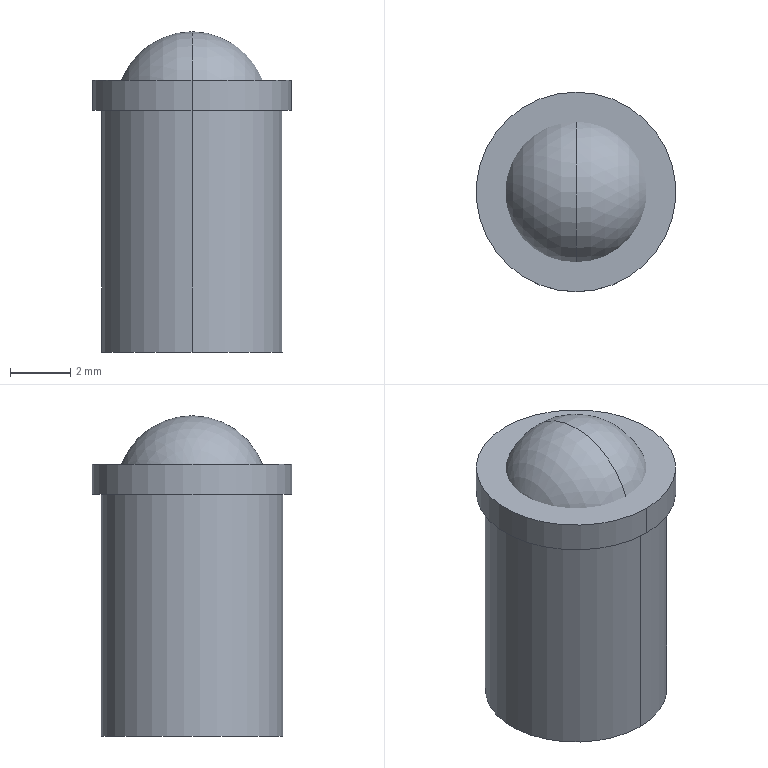Part | STEP file | 22DDSceondZAL02-M6_Default | 2 solids | 9 faces | box 6.6 x 6.6 x 10.6 mm | volume 325.856 mm3 | cylinder 4 | plane 3 | sphere 2 | commonest cylinder face diameters 6 x2 6.6 x2
STEP:
#1=CARTESIAN_POINT('',(0.,0.,0.));
#2=DIRECTION('',(0.,0.,1.));
#3=DIRECTION('',(1.,0.,0.));
#4=AXIS2_PLACEMENT_3D('',#1,#2,#3);
#5=CARTESIAN_POINT('',(0.,3.,-1.));
#6=VERTEX_POINT('',#5);
#7=CARTESIAN_POINT('',(0.,-3.,-1.));
#8=VERTEX_POINT('',#7);
#9=CARTESIAN_POINT('',(0.,0.,-1.));
#10=DIRECTION('',(0.,0.,-1.));
#11=DIRECTION('',(0.,1.,0.));
#12=AXIS2_PLACEMENT_3D('',#9,#10,#11);
#13=CIRCLE('',#12,3.);
#14=CARTESIAN_POINT('',(0.,0.,-9.));
#15=DIRECTION('',(0.,0.,-1.));
#16=DIRECTION('',(0.,1.,0.));
#17=AXIS2_PLACEMENT_3D('',#14,#15,#16);
#18=CYLINDRICAL_SURFACE('',#17,3.);
#19=CARTESIAN_POINT('',(0.,-8.));
#20=DIRECTION('',(1.,0.));
#21=VECTOR('',#20,1.);
#22=LINE('',#19,#21);
#23=(GEOMETRIC_REPRESENTATION_CONTEXT(2)PARAMETRIC_REPRESENTATION_CONTEXT()REPRESENTATION_CONTEXT('',''));
#24=DEFINITIONAL_REPRESENTATION('',(#22),#23);
#25=PCURVE('',#18,#24);
#26=CARTESIAN_POINT('',(0.,3.3,-1.));
#27=DIRECTION('',(0.,0.,-1.));
#28=DIRECTION('',(0.,1.,0.));
#29=AXIS2_PLACEMENT_3D('',#26,#27,#28);
#30=PLANE('',#29);
#31=CARTESIAN_POINT('',(-3.3,0.));
#32=DIRECTION('',(1.,0.));
#33=AXIS2_PLACEMENT_2D('',#31,#32);
#34=CIRCLE('',#33,3.);
#35=(GEOMETRIC_REPRESENTATION_CONTEXT(2)PARAMETRIC_REPRESENTATION_CONTEXT()REPRESENTATION_CONTEXT('',''));
#36=DEFINITIONAL_REPRESENTATION('',(#34),#35);
#37=PCURVE('',#30,#36);
#38=SURFACE_CURVE('',#13,(#25,#37),.PCURVE_S1.);
#39=EDGE_CURVE('',#6,#8,#38,.T.);
#40=ORIENTED_EDGE('',*,*,#39,.T.);
#41=CARTESIAN_POINT('',(0.,-3.,-9.));
#42=VERTEX_POINT('',#41);
#43=CARTESIAN_POINT('',(0.,-3.,-9.));
#44=DIRECTION('',(0.,0.,-1.));
#45=VECTOR('',#44,1.);
#46=LINE('',#43,#45);
#47=CARTESIAN_POINT('',(3.142,0.));
#48=DIRECTION('',(0.,1.));
#49=VECTOR('',#48,1.);
#50=LINE('',#47,#49);
#51=(GEOMETRIC_REPRESENTATION_CONTEXT(2)PARAMETRIC_REPRESENTATION_CONTEXT()REPRESENTATION_CONTEXT('',''));
#52=DEFINITIONAL_REPRESENTATION('',(#50),#51);
#53=PCURVE('',#18,#52);
#54=CARTESIAN_POINT('',(0.,0.,-9.));
#55=DIRECTION('',(0.,0.,-1.));
#56=DIRECTION('',(0.,1.,0.));
#57=AXIS2_PLACEMENT_3D('',#54,#55,#56);
#58=CYLINDRICAL_SURFACE('',#57,3.);
#59=CARTESIAN_POINT('',(3.142,0.));
#60=DIRECTION('',(0.,1.));
#61=VECTOR('',#60,1.);
#62=LINE('',#59,#61);
#63=(GEOMETRIC_REPRESENTATION_CONTEXT(2)PARAMETRIC_REPRESENTATION_CONTEXT()REPRESENTATION_CONTEXT('',''));
#64=DEFINITIONAL_REPRESENTATION('',(#62),#63);
#65=PCURVE('',#58,#64);
#66=SURFACE_CURVE('',#46,(#53,#65),.PCURVE_S1.);
#67=EDGE_CURVE('',#8,#42,#66,.T.);
#68=ORIENTED_EDGE('',*,*,#67,.T.);
#69=CARTESIAN_POINT('',(0.,3.,-9.));
#70=VERTEX_POINT('',#69);
#71=CARTESIAN_POINT('',(0.,0.,-9.));
#72=DIRECTION('',(0.,0.,-1.));
#73=DIRECTION('',(0.,1.,0.));
#74=AXIS2_PLACEMENT_3D('',#71,#72,#73);
#75=CIRCLE('',#74,3.);
#76=CARTESIAN_POINT('',(0.,0.));
#77=DIRECTION('',(1.,0.));
#78=VECTOR('',#77,1.);
#79=LINE('',#76,#78);
#80=(GEOMETRIC_REPRESENTATION_CONTEXT(2)PARAMETRIC_REPRESENTATION_CONTEXT()REPRESENTATION_CONTEXT('',''));
#81=DEFINITIONAL_REPRESENTATION('',(#79),#80);
#82=PCURVE('',#18,#81);
#83=CARTESIAN_POINT('',(0.,3.,-9.));
#84=DIRECTION('',(0.,0.,-1.));
#85=DIRECTION('',(0.,1.,0.));
#86=AXIS2_PLACEMENT_3D('',#83,#84,#85);
#87=PLANE('',#86);
#88=CARTESIAN_POINT('',(-3.,0.));
#89=DIRECTION('',(1.,0.));
#90=AXIS2_PLACEMENT_2D('',#88,#89);
#91=CIRCLE('',#90,3.);
#92=(GEOMETRIC_REPRESENTATION_CONTEXT(2)PARAMETRIC_REPRESENTATION_CONTEXT()REPRESENTATION_CONTEXT('',''));
#93=DEFINITIONAL_REPRESENTATION('',(#91),#92);
#94=PCURVE('',#87,#93);
#95=SURFACE_CURVE('',#75,(#82,#94),.PCURVE_S1.);
#96=EDGE_CURVE('',#70,#42,#95,.T.);
#97=ORIENTED_EDGE('',*,*,#96,.F.);
#98=CARTESIAN_POINT('',(0.,3.,-9.));
#99=DIRECTION('',(0.,0.,-1.));
#100=VECTOR('',#99,1.);
#101=LINE('',#98,#100);
#102=CARTESIAN_POINT('',(0.,0.));
#103=DIRECTION('',(0.,1.));
#104=VECTOR('',#103,1.);
#105=LINE('',#102,#104);
#106=(GEOMETRIC_REPRESENTATION_CONTEXT(2)PARAMETRIC_REPRESENTATION_CONTEXT()REPRESENTATION_CONTEXT('',''));
#107=DEFINITIONAL_REPRESENTATION('',(#105),#106);
#108=PCURVE('',#18,#107);
#109=CARTESIAN_POINT('',(6.283,0.));
#110=DIRECTION('',(0.,1.));
#111=VECTOR('',#110,1.);
#112=LINE('',#109,#111);
#113=(GEOMETRIC_REPRESENTATION_CONTEXT(2)PARAMETRIC_REPRESENTATION_CONTEXT()REPRESENTATION_CONTEXT('',''));
#114=DEFINITIONAL_REPRESENTATION('',(#112),#113);
#115=PCURVE('',#58,#114);
#116=SURFACE_CURVE('',#101,(#108,#115),.PCURVE_S1.);
#117=EDGE_CURVE('',#6,#70,#116,.T.);
#118=ORIENTED_EDGE('',*,*,#117,.F.);
#119=EDGE_LOOP('',(#40,#68,#97,#118));
#120=FACE_BOUND('',#119,.T.);
#121=ADVANCED_FACE('',(#120),#18,.T.);
#122=CARTESIAN_POINT('',(0.,3.3,0.));
#123=VERTEX_POINT('',#122);
#124=CARTESIAN_POINT('',(0.,-3.3,0.));
#125=VERTEX_POINT('',#124);
#126=CARTESIAN_POINT('',(0.,0.,0.));
#127=DIRECTION('',(0.,0.,-1.));
#128=DIRECTION('',(0.,1.,0.));
#129=AXIS2_PLACEMENT_3D('',#126,#127,#128);
#130=CIRCLE('',#129,3.3);
#131=CARTESIAN_POINT('',(0.,0.,-9.));
#132=DIRECTION('',(0.,0.,-1.));
#133=DIRECTION('',(0.,1.,0.));
#134=AXIS2_PLACEMENT_3D('',#131,#132,#133);
#135=CYLINDRICAL_SURFACE('',#134,3.3);
#136=CARTESIAN_POINT('',(0.,-9.));
#137=DIRECTION('',(1.,0.));
#138=VECTOR('',#137,1.);
#139=LINE('',#136,#138);
#140=(GEOMETRIC_REPRESENTATION_CONTEXT(2)PARAMETRIC_REPRESENTATION_CONTEXT()REPRESENTATION_CONTEXT('',''));
#141=DEFINITIONAL_REPRESENTATION('',(#139),#140);
#142=PCURVE('',#135,#141);
#143=CARTESIAN_POINT('',(0.,0.,0.));
#144=DIRECTION('',(0.,0.,1.));
#145=DIRECTION('',(0.,-1.,0.));
#146=AXIS2_PLACEMENT_3D('',#143,#144,#145);
#147=PLANE('',#146);
#148=CARTESIAN_POINT('',(-3.3,0.));
#149=CARTESIAN_POINT('',(-3.3,5.716));
#150=CARTESIAN_POINT('',(1.65,2.858));
#151=CARTESIAN_POINT('',(6.6,0.));
#152=CARTESIAN_POINT('',(1.65,-2.858));
#153=CARTESIAN_POINT('',(-3.3,-5.716));
#154=CARTESIAN_POINT('',(-3.3,0.));
#155=(BOUNDED_CURVE()B_SPLINE_CURVE(2,(#148,#149,#150,#151,#152,#153,#154),.UNSPECIFIED.,.T.,.F.)B_SPLINE_CURVE_WITH_KNOTS((1,2,2,2,2,1),(-2.094,0.,2.094,4.189,6.283,8.378),.UNSPECIFIED.)CURVE()GEOMETRIC_REPRESENTATION_ITEM()RATIONAL_B_SPLINE_CURVE((1.,0.5,1.,0.5,1.,0.5,1.))REPRESENTATION_ITEM(''));
#156=(GEOMETRIC_REPRESENTATION_CONTEXT(2)PARAMETRIC_REPRESENTATION_CONTEXT()REPRESENTATION_CONTEXT('',''));
#157=DEFINITIONAL_REPRESENTATION('',(#155),#156);
#158=PCURVE('',#147,#157);
#159=SURFACE_CURVE('',#130,(#142,#158),.PCURVE_S1.);
#160=EDGE_CURVE('',#123,#125,#159,.T.);
#161=ORIENTED_EDGE('',*,*,#160,.T.);
#162=CARTESIAN_POINT('',(0.,-3.3,-1.));
#163=VERTEX_POINT('',#162);
#164=CARTESIAN_POINT('',(0.,-3.3,-9.));
#165=DIRECTION('',(0.,0.,-1.));
#166=VECTOR('',#165,1.);
#167=LINE('',#164,#166);
#168=CARTESIAN_POINT('',(3.142,0.));
#169=DIRECTION('',(0.,1.));
#170=VECTOR('',#169,1.);
#171=LINE('',#168,#170);
#172=(GEOMETRIC_REPRESENTATION_CONTEXT(2)PARAMETRIC_REPRESENTATION_CONTEXT()REPRESENTATION_CONTEXT('',''));
#173=DEFINITIONAL_REPRESENTATION('',(#171),#172);
#174=PCURVE('',#135,#173);
#175=CARTESIAN_POINT('',(0.,0.,-9.));
#176=DIRECTION('',(0.,0.,-1.));
#177=DIRECTION('',(0.,1.,0.));
#178=AXIS2_PLACEMENT_3D('',#175,#176,#177);
#179=CYLINDRICAL_SURFACE('',#178,3.3);
#180=CARTESIAN_POINT('',(3.142,0.));
#181=DIRECTION('',(0.,1.));
#182=VECTOR('',#181,1.);
#183=LINE('',#180,#182);
#184=(GEOMETRIC_REPRESENTATION_CONTEXT(2)PARAMETRIC_REPRESENTATION_CONTEXT()REPRESENTATION_CONTEXT('',''));
#185=DEFINITIONAL_REPRESENTATION('',(#183),#184);
#186=PCURVE('',#179,#185);
#187=SURFACE_CURVE('',#167,(#174,#186),.PCURVE_S1.);
#188=EDGE_CURVE('',#125,#163,#187,.T.);
#189=ORIENTED_EDGE('',*,*,#188,.T.);
#190=CARTESIAN_POINT('',(0.,3.3,-1.));
#191=VERTEX_POINT('',#190);
#192=CARTESIAN_POINT('',(0.,0.,-1.));
#193=DIRECTION('',(0.,0.,-1.));
#194=DIRECTION('',(0.,1.,0.));
#195=AXIS2_PLACEMENT_3D('',#192,#193,#194);
#196=CIRCLE('',#195,3.3);
#197=CARTESIAN_POINT('',(0.,-8.));
#198=DIRECTION('',(1.,0.));
#199=VECTOR('',#198,1.);
#200=LINE('',#197,#199);
#201=(GEOMETRIC_REPRESENTATION_CONTEXT(2)PARAMETRIC_REPRESENTATION_CONTEXT()REPRESENTATION_CONTEXT('',''));
#202=DEFINITIONAL_REPRESENTATION('',(#200),#201);
#203=PCURVE('',#135,#202);
#204=CARTESIAN_POINT('',(-3.3,0.));
#205=DIRECTION('',(1.,0.));
#206=AXIS2_PLACEMENT_2D('',#204,#205);
#207=CIRCLE('',#206,3.3);
#208=(GEOMETRIC_REPRESENTATION_CONTEXT(2)PARAMETRIC_REPRESENTATION_CONTEXT()REPRESENTATION_CONTEXT('',''));
#209=DEFINITIONAL_REPRESENTATION('',(#207),#208);
#210=PCURVE('',#30,#209);
#211=SURFACE_CURVE('',#196,(#203,#210),.PCURVE_S1.);
#212=EDGE_CURVE('',#191,#163,#211,.T.);
#213=ORIENTED_EDGE('',*,*,#212,.F.);
#214=CARTESIAN_POINT('',(0.,3.3,-9.));
#215=DIRECTION('',(0.,0.,-1.));
#216=VECTOR('',#215,1.);
#217=LINE('',#214,#216);
#218=CARTESIAN_POINT('',(0.,0.));
#219=DIRECTION('',(0.,1.));
#220=VECTOR('',#219,1.);
#221=LINE('',#218,#220);
#222=(GEOMETRIC_REPRESENTATION_CONTEXT(2)PARAMETRIC_REPRESENTATION_CONTEXT()REPRESENTATION_CONTEXT('',''));
#223=DEFINITIONAL_REPRESENTATION('',(#221),#222);
#224=PCURVE('',#135,#223);
#225=CARTESIAN_POINT('',(6.283,0.));
#226=DIRECTION('',(0.,1.));
#227=VECTOR('',#226,1.);
#228=LINE('',#225,#227);
#229=(GEOMETRIC_REPRESENTATION_CONTEXT(2)PARAMETRIC_REPRESENTATION_CONTEXT()REPRESENTATION_CONTEXT('',''));
#230=DEFINITIONAL_REPRESENTATION('',(#228),#229);
#231=PCURVE('',#179,#230);
#232=SURFACE_CURVE('',#217,(#224,#231),.PCURVE_S1.);
#233=EDGE_CURVE('',#123,#191,#232,.T.);
#234=ORIENTED_EDGE('',*,*,#233,.F.);
#235=EDGE_LOOP('',(#161,#189,#213,#234));
#236=FACE_BOUND('',#235,.T.);
#237=ADVANCED_FACE('',(#236),#135,.T.);
#238=ORIENTED_EDGE('',*,*,#188,.F.);
#239=CARTESIAN_POINT('',(0.,0.,0.));
#240=DIRECTION('',(0.,0.,-1.));
#241=DIRECTION('',(0.,1.,0.));
#242=AXIS2_PLACEMENT_3D('',#239,#240,#241);
#243=CIRCLE('',#242,3.3);
#244=CARTESIAN_POINT('',(0.,-9.));
#245=DIRECTION('',(1.,0.));
#246=VECTOR('',#245,1.);
#247=LINE('',#244,#246);
#248=(GEOMETRIC_REPRESENTATION_CONTEXT(2)PARAMETRIC_REPRESENTATION_CONTEXT()REPRESENTATION_CONTEXT('',''));
#249=DEFINITIONAL_REPRESENTATION('',(#247),#248);
#250=PCURVE('',#179,#249);
#251=CARTESIAN_POINT('',(-3.3,0.));
#252=CARTESIAN_POINT('',(-3.3,5.716));
#253=CARTESIAN_POINT('',(1.65,2.858));
#254=CARTESIAN_POINT('',(6.6,0.));
#255=CARTESIAN_POINT('',(1.65,-2.858));
#256=CARTESIAN_POINT('',(-3.3,-5.716));
#257=CARTESIAN_POINT('',(-3.3,0.));
#258=(BOUNDED_CURVE()B_SPLINE_CURVE(2,(#251,#252,#253,#254,#255,#256,#257),.UNSPECIFIED.,.T.,.F.)B_SPLINE_CURVE_WITH_KNOTS((1,2,2,2,2,1),(-2.094,0.,2.094,4.189,6.283,8.378),.UNSPECIFIED.)CURVE()GEOMETRIC_REPRESENTATION_ITEM()RATIONAL_B_SPLINE_CURVE((1.,0.5,1.,0.5,1.,0.5,1.))REPRESENTATION_ITEM(''));
#259=(GEOMETRIC_REPRESENTATION_CONTEXT(2)PARAMETRIC_REPRESENTATION_CONTEXT()REPRESENTATION_CONTEXT('',''));
#260=DEFINITIONAL_REPRESENTATION('',(#258),#259);
#261=PCURVE('',#147,#260);
#262=SURFACE_CURVE('',#243,(#250,#261),.PCURVE_S1.);
#263=EDGE_CURVE('',#125,#123,#262,.T.);
#264=ORIENTED_EDGE('',*,*,#263,.T.);
#265=ORIENTED_EDGE('',*,*,#233,.T.);
#266=CARTESIAN_POINT('',(0.,0.,-1.));
#267=DIRECTION('',(0.,0.,-1.));
#268=DIRECTION('',(0.,1.,0.));
#269=AXIS2_PLACEMENT_3D('',#266,#267,#268);
#270=CIRCLE('',#269,3.3);
#271=CARTESIAN_POINT('',(0.,-8.));
#272=DIRECTION('',(1.,0.));
#273=VECTOR('',#272,1.);
#274=LINE('',#271,#273);
#275=(GEOMETRIC_REPRESENTATION_CONTEXT(2)PARAMETRIC_REPRESENTATION_CONTEXT()REPRESENTATION_CONTEXT('',''));
#276=DEFINITIONAL_REPRESENTATION('',(#274),#275);
#277=PCURVE('',#179,#276);
#278=CARTESIAN_POINT('',(-3.3,0.));
#279=DIRECTION('',(1.,0.));
#280=AXIS2_PLACEMENT_2D('',#278,#279);
#281=CIRCLE('',#280,3.3);
#282=(GEOMETRIC_REPRESENTATION_CONTEXT(2)PARAMETRIC_REPRESENTATION_CONTEXT()REPRESENTATION_CONTEXT('',''));
#283=DEFINITIONAL_REPRESENTATION('',(#281),#282);
#284=PCURVE('',#30,#283);
#285=SURFACE_CURVE('',#270,(#277,#284),.PCURVE_S1.);
#286=EDGE_CURVE('',#163,#191,#285,.T.);
#287=ORIENTED_EDGE('',*,*,#286,.F.);
#288=EDGE_LOOP('',(#238,#264,#265,#287));
#289=FACE_BOUND('',#288,.T.);
#290=ADVANCED_FACE('',(#289),#179,.T.);
#291=ORIENTED_EDGE('',*,*,#212,.T.);
#292=ORIENTED_EDGE('',*,*,#286,.T.);
#293=EDGE_LOOP('',(#291,#292));
#294=FACE_BOUND('',#293,.T.);
#295=ORIENTED_EDGE('',*,*,#39,.F.);
#296=CARTESIAN_POINT('',(0.,0.,-1.));
#297=DIRECTION('',(0.,0.,-1.));
#298=DIRECTION('',(0.,1.,0.));
#299=AXIS2_PLACEMENT_3D('',#296,#297,#298);
#300=CIRCLE('',#299,3.);
#301=CARTESIAN_POINT('',(-3.3,0.));
#302=DIRECTION('',(1.,0.));
#303=AXIS2_PLACEMENT_2D('',#301,#302);
#304=CIRCLE('',#303,3.);
#305=(GEOMETRIC_REPRESENTATION_CONTEXT(2)PARAMETRIC_REPRESENTATION_CONTEXT()REPRESENTATION_CONTEXT('',''));
#306=DEFINITIONAL_REPRESENTATION('',(#304),#305);
#307=PCURVE('',#30,#306);
#308=CARTESIAN_POINT('',(0.,-8.));
#309=DIRECTION('',(1.,0.));
#310=VECTOR('',#309,1.);
#311=LINE('',#308,#310);
#312=(GEOMETRIC_REPRESENTATION_CONTEXT(2)PARAMETRIC_REPRESENTATION_CONTEXT()REPRESENTATION_CONTEXT('',''));
#313=DEFINITIONAL_REPRESENTATION('',(#311),#312);
#314=PCURVE('',#58,#313);
#315=SURFACE_CURVE('',#300,(#307,#314),.PCURVE_S1.);
#316=EDGE_CURVE('',#8,#6,#315,.T.);
#317=ORIENTED_EDGE('',*,*,#316,.F.);
#318=EDGE_LOOP('',(#295,#317));
#319=FACE_BOUND('',#318,.T.);
#320=ADVANCED_FACE('',(#294,#319),#30,.T.);
#321=ORIENTED_EDGE('',*,*,#67,.F.);
#322=ORIENTED_EDGE('',*,*,#316,.T.);
#323=ORIENTED_EDGE('',*,*,#117,.T.);
#324=CARTESIAN_POINT('',(0.,0.,-9.));
#325=DIRECTION('',(0.,0.,-1.));
#326=DIRECTION('',(0.,1.,0.));
#327=AXIS2_PLACEMENT_3D('',#324,#325,#326);
#328=CIRCLE('',#327,3.);
#329=CARTESIAN_POINT('',(0.,0.));
#330=DIRECTION('',(1.,0.));
#331=VECTOR('',#330,1.);
#332=LINE('',#329,#331);
#333=(GEOMETRIC_REPRESENTATION_CONTEXT(2)PARAMETRIC_REPRESENTATION_CONTEXT()REPRESENTATION_CONTEXT('',''));
#334=DEFINITIONAL_REPRESENTATION('',(#332),#333);
#335=PCURVE('',#58,#334);
#336=CARTESIAN_POINT('',(-3.,0.));
#337=DIRECTION('',(1.,0.));
#338=AXIS2_PLACEMENT_2D('',#336,#337);
#339=CIRCLE('',#338,3.);
#340=(GEOMETRIC_REPRESENTATION_CONTEXT(2)PARAMETRIC_REPRESENTATION_CONTEXT()REPRESENTATION_CONTEXT('',''));
#341=DEFINITIONAL_REPRESENTATION('',(#339),#340);
#342=PCURVE('',#87,#341);
#343=SURFACE_CURVE('',#328,(#335,#342),.PCURVE_S1.);
#344=EDGE_CURVE('',#42,#70,#343,.T.);
#345=ORIENTED_EDGE('',*,*,#344,.F.);
#346=EDGE_LOOP('',(#321,#322,#323,#345));
#347=FACE_BOUND('',#346,.T.);
#348=ADVANCED_FACE('',(#347),#58,.T.);
#349=ORIENTED_EDGE('',*,*,#96,.T.);
#350=ORIENTED_EDGE('',*,*,#344,.T.);
#351=EDGE_LOOP('',(#349,#350));
#352=FACE_BOUND('',#351,.T.);
#353=ADVANCED_FACE('',(#352),#87,.T.);
#354=ORIENTED_EDGE('',*,*,#160,.F.);
#355=ORIENTED_EDGE('',*,*,#263,.F.);
#356=EDGE_LOOP('',(#354,#355));
#357=FACE_BOUND('',#356,.T.);
#358=ADVANCED_FACE('',(#357),#147,.T.);
#359=CLOSED_SHELL('',(#121,#237,#290,#320,#348,#353,#358));
#360=MANIFOLD_SOLID_BREP('',#359);
#361=CARTESIAN_POINT('',(0.,2.5,-0.9));
#362=VERTEX_POINT('',#361);
#363=CARTESIAN_POINT('',(0.,0.,1.6));
#364=VERTEX_POINT('',#363);
#365=CARTESIAN_POINT('',(0.,0.,-0.9));
#366=DIRECTION('',(1.,0.,0.));
#367=DIRECTION('',(0.,0.,-1.));
#368=AXIS2_PLACEMENT_3D('',#365,#366,#367);
#369=CIRCLE('',#368,2.5);
#370=CARTESIAN_POINT('',(0.,0.,-0.9));
#371=DIRECTION('',(-1.,0.,0.));
#372=DIRECTION('',(0.,1.,0.));
#373=AXIS2_PLACEMENT_3D('',#370,#371,#372);
#374=SPHERICAL_SURFACE('',#373,2.5);
#375=CARTESIAN_POINT('',(7.854,0.));
#376=CARTESIAN_POINT('',(7.806,0.));
#377=CARTESIAN_POINT('',(7.711,0.));
#378=CARTESIAN_POINT('',(7.568,0.));
#379=CARTESIAN_POINT('',(7.426,0.));
#380=CARTESIAN_POINT('',(7.283,0.));
#381=CARTESIAN_POINT('',(7.14,0.));
#382=CARTESIAN_POINT('',(6.997,0.));
#383=CARTESIAN_POINT('',(6.854,0.));
#384=CARTESIAN_POINT('',(6.712,0.));
#385=CARTESIAN_POINT('',(6.569,0.));
#386=CARTESIAN_POINT('',(6.426,0.));
#387=CARTESIAN_POINT('',(6.283,0.));
#388=CARTESIAN_POINT('',(6.14,0.));
#389=CARTESIAN_POINT('',(5.998,0.));
#390=CARTESIAN_POINT('',(5.855,0.));
#391=CARTESIAN_POINT('',(5.712,0.));
#392=CARTESIAN_POINT('',(5.569,0.));
#393=CARTESIAN_POINT('',(5.426,0.));
#394=CARTESIAN_POINT('',(5.284,0.));
#395=CARTESIAN_POINT('',(5.141,0.));
#396=CARTESIAN_POINT('',(4.998,0.));
#397=CARTESIAN_POINT('',(4.855,0.));
#398=CARTESIAN_POINT('',(4.76,0.));
#399=CARTESIAN_POINT('',(4.712,0.));
#400=B_SPLINE_CURVE_WITH_KNOTS('',3,(#375,#376,#377,#378,#379,#380,#381,#382,#383,#384,#385,#386,#387,#388,#389,#390,#391,#392,#393,#394,#395,#396,#397,#398,#399),.UNSPECIFIED.,.F.,.F.,(4,1,1,1,1,1,1,1,1,1,1,1,1,1,1,1,1,1,1,1,1,1,4),(0.,0.1428,0.2856,0.4284,0.5712,0.714,0.8568,0.9996,1.142,1.285,1.428,1.571,1.714,1.856,1.999,2.142,2.285,2.428,2.57,2.713,2.856,2.999,3.142),.QUASI_UNIFORM_KNOTS.);
#401=(GEOMETRIC_REPRESENTATION_CONTEXT(2)PARAMETRIC_REPRESENTATION_CONTEXT()REPRESENTATION_CONTEXT('',''));
#402=DEFINITIONAL_REPRESENTATION('',(#400),#401);
#403=PCURVE('',#374,#402);
#404=CARTESIAN_POINT('',(0.,0.,-0.9));
#405=DIRECTION('',(-1.,0.,0.));
#406=DIRECTION('',(0.,1.,0.));
#407=AXIS2_PLACEMENT_3D('',#404,#405,#406);
#408=SPHERICAL_SURFACE('',#407,2.5);
#409=CARTESIAN_POINT('',(6.283,0.));
#410=CARTESIAN_POINT('',(6.259,0.));
#411=CARTESIAN_POINT('',(6.212,0.));
#412=CARTESIAN_POINT('',(6.14,0.));
#413=CARTESIAN_POINT('',(6.069,0.));
#414=CARTESIAN_POINT('',(5.998,0.));
#415=CARTESIAN_POINT('',(5.926,0.));
#416=CARTESIAN_POINT('',(5.855,0.));
#417=CARTESIAN_POINT('',(5.783,0.));
#418=CARTESIAN_POINT('',(5.712,0.));
#419=CARTESIAN_POINT('',(5.641,0.));
#420=CARTESIAN_POINT('',(5.569,0.));
#421=CARTESIAN_POINT('',(5.498,0.));
#422=CARTESIAN_POINT('',(5.426,0.));
#423=CARTESIAN_POINT('',(5.355,0.));
#424=CARTESIAN_POINT('',(5.284,0.));
#425=CARTESIAN_POINT('',(5.212,0.));
#426=CARTESIAN_POINT('',(5.141,0.));
#427=CARTESIAN_POINT('',(5.069,0.));
#428=CARTESIAN_POINT('',(4.998,0.));
#429=CARTESIAN_POINT('',(4.927,0.));
#430=CARTESIAN_POINT('',(4.855,0.));
#431=CARTESIAN_POINT('',(4.784,0.));
#432=CARTESIAN_POINT('',(4.736,0.));
#433=CARTESIAN_POINT('',(4.712,0.));
#434=B_SPLINE_CURVE_WITH_KNOTS('',3,(#409,#410,#411,#412,#413,#414,#415,#416,#417,#418,#419,#420,#421,#422,#423,#424,#425,#426,#427,#428,#429,#430,#431,#432,#433),.UNSPECIFIED.,.F.,.F.,(4,1,1,1,1,1,1,1,1,1,1,1,1,1,1,1,1,1,1,1,1,1,4),(1.571,1.642,1.714,1.785,1.856,1.928,1.999,2.071,2.142,2.213,2.285,2.356,2.428,2.499,2.57,2.642,2.713,2.785,2.856,2.927,2.999,3.07,3.142),.QUASI_UNIFORM_KNOTS.);
#435=(GEOMETRIC_REPRESENTATION_CONTEXT(2)PARAMETRIC_REPRESENTATION_CONTEXT()REPRESENTATION_CONTEXT('',''));
#436=DEFINITIONAL_REPRESENTATION('',(#434),#435);
#437=PCURVE('',#408,#436);
#438=SURFACE_CURVE('',#369,(#403,#437),.PCURVE_S1.);
#439=EDGE_CURVE('',#362,#364,#438,.T.);
#440=ORIENTED_EDGE('',*,*,#439,.F.);
#441=CARTESIAN_POINT('',(-2.5,0.,-0.9));
#442=VERTEX_POINT('',#441);
#443=CARTESIAN_POINT('',(0.,2.5,-0.9));
#444=CARTESIAN_POINT('',(-0.6545,2.5,-0.9));
#445=CARTESIAN_POINT('',(-1.309,2.294,-0.9));
#446=CARTESIAN_POINT('',(-1.883,1.883,-0.9));
#447=CARTESIAN_POINT('',(-2.294,1.309,-0.9));
#448=CARTESIAN_POINT('',(-2.5,0.6545,-0.9));
#449=CARTESIAN_POINT('',(-2.5,0.,-0.9));
#450=B_SPLINE_CURVE_WITH_KNOTS('',6,(#443,#444,#445,#446,#447,#448,#449),.UNSPECIFIED.,.F.,.F.,(7,7),(0.,1.571),.PIECEWISE_BEZIER_KNOTS.);
#451=CARTESIAN_POINT('',(6.283,0.));
#452=DIRECTION('',(0.,1.));
#453=VECTOR('',#452,1.);
#454=LINE('',#451,#453);
#455=(GEOMETRIC_REPRESENTATION_CONTEXT(2)PARAMETRIC_REPRESENTATION_CONTEXT()REPRESENTATION_CONTEXT('',''));
#456=DEFINITIONAL_REPRESENTATION('',(#454),#455);
#457=PCURVE('',#374,#456);
#458=CARTESIAN_POINT('',(0.,0.));
#459=DIRECTION('',(0.,1.));
#460=VECTOR('',#459,1.);
#461=LINE('',#458,#460);
#462=(GEOMETRIC_REPRESENTATION_CONTEXT(2)PARAMETRIC_REPRESENTATION_CONTEXT()REPRESENTATION_CONTEXT('',''));
#463=DEFINITIONAL_REPRESENTATION('',(#461),#462);
#464=PCURVE('',#374,#463);
#465=SEAM_CURVE('',#450,(#457,#464),.PCURVE_S1.);
#466=EDGE_CURVE('',#362,#442,#465,.T.);
#467=ORIENTED_EDGE('',*,*,#466,.T.);
#468=ORIENTED_EDGE('',*,*,#466,.F.);
#469=CARTESIAN_POINT('',(0.,0.,-3.4));
#470=VERTEX_POINT('',#469);
#471=CARTESIAN_POINT('',(0.,0.,-0.9));
#472=DIRECTION('',(1.,0.,0.));
#473=DIRECTION('',(0.,0.,-1.));
#474=AXIS2_PLACEMENT_3D('',#471,#472,#473);
#475=CIRCLE('',#474,2.5);
#476=CARTESIAN_POINT('',(1.571,0.));
#477=CARTESIAN_POINT('',(1.523,0.));
#478=CARTESIAN_POINT('',(1.428,0.));
#479=CARTESIAN_POINT('',(1.285,0.));
#480=CARTESIAN_POINT('',(1.142,0.));
#481=CARTESIAN_POINT('',(0.9996,0.));
#482=CARTESIAN_POINT('',(0.8568,0.));
#483=CARTESIAN_POINT('',(0.714,0.));
#484=CARTESIAN_POINT('',(0.5712,0.));
#485=CARTESIAN_POINT('',(0.4284,0.));
#486=CARTESIAN_POINT('',(0.2856,0.));
#487=CARTESIAN_POINT('',(0.1428,0.));
#488=CARTESIAN_POINT('',(0.,0.));
#489=CARTESIAN_POINT('',(-0.1428,0.));
#490=CARTESIAN_POINT('',(-0.2856,0.));
#491=CARTESIAN_POINT('',(-0.4284,0.));
#492=CARTESIAN_POINT('',(-0.5712,0.));
#493=CARTESIAN_POINT('',(-0.714,0.));
#494=CARTESIAN_POINT('',(-0.8568,0.));
#495=CARTESIAN_POINT('',(-0.9996,0.));
#496=CARTESIAN_POINT('',(-1.142,0.));
#497=CARTESIAN_POINT('',(-1.285,0.));
#498=CARTESIAN_POINT('',(-1.428,0.));
#499=CARTESIAN_POINT('',(-1.523,0.));
#500=CARTESIAN_POINT('',(-1.571,0.));
#501=B_SPLINE_CURVE_WITH_KNOTS('',3,(#476,#477,#478,#479,#480,#481,#482,#483,#484,#485,#486,#487,#488,#489,#490,#491,#492,#493,#494,#495,#496,#497,#498,#499,#500),.UNSPECIFIED.,.F.,.F.,(4,1,1,1,1,1,1,1,1,1,1,1,1,1,1,1,1,1,1,1,1,1,4),(0.,0.1428,0.2856,0.4284,0.5712,0.714,0.8568,0.9996,1.142,1.285,1.428,1.571,1.714,1.856,1.999,2.142,2.285,2.428,2.57,2.713,2.856,2.999,3.142),.QUASI_UNIFORM_KNOTS.);
#502=(GEOMETRIC_REPRESENTATION_CONTEXT(2)PARAMETRIC_REPRESENTATION_CONTEXT()REPRESENTATION_CONTEXT('',''));
#503=DEFINITIONAL_REPRESENTATION('',(#501),#502);
#504=PCURVE('',#374,#503);
#505=CARTESIAN_POINT('',(1.571,0.));
#506=DIRECTION('',(-1.,0.));
#507=VECTOR('',#506,1.);
#508=LINE('',#505,#507);
#509=(GEOMETRIC_REPRESENTATION_CONTEXT(2)PARAMETRIC_REPRESENTATION_CONTEXT()REPRESENTATION_CONTEXT('',''));
#510=DEFINITIONAL_REPRESENTATION('',(#508),#509);
#511=PCURVE('',#408,#510);
#512=SURFACE_CURVE('',#475,(#504,#511),.PCURVE_S1.);
#513=EDGE_CURVE('',#470,#362,#512,.T.);
#514=ORIENTED_EDGE('',*,*,#513,.F.);
#515=CARTESIAN_POINT('',(0.,0.,-0.9));
#516=DIRECTION('',(-1.,0.,0.));
#517=DIRECTION('',(0.,-1.,0.));
#518=AXIS2_PLACEMENT_3D('',#515,#516,#517);
#519=CIRCLE('',#518,2.5);
#520=CARTESIAN_POINT('',(-3.142,0.));
#521=DIRECTION('',(1.,0.));
#522=VECTOR('',#521,1.);
#523=LINE('',#520,#522);
#524=(GEOMETRIC_REPRESENTATION_CONTEXT(2)PARAMETRIC_REPRESENTATION_CONTEXT()REPRESENTATION_CONTEXT('',''));
#525=DEFINITIONAL_REPRESENTATION('',(#523),#524);
#526=PCURVE('',#374,#525);
#527=CARTESIAN_POINT('',(-3.142,0.));
#528=DIRECTION('',(1.,0.));
#529=VECTOR('',#528,1.);
#530=LINE('',#527,#529);
#531=(GEOMETRIC_REPRESENTATION_CONTEXT(2)PARAMETRIC_REPRESENTATION_CONTEXT()REPRESENTATION_CONTEXT('',''));
#532=DEFINITIONAL_REPRESENTATION('',(#530),#531);
#533=PCURVE('',#408,#532);
#534=SURFACE_CURVE('',#519,(#526,#533),.PCURVE_S1.);
#535=EDGE_CURVE('',#470,#364,#534,.T.);
#536=ORIENTED_EDGE('',*,*,#535,.T.);
#537=EDGE_LOOP('',(#440,#467,#468,#514,#536));
#538=FACE_BOUND('',#537,.T.);
#539=ADVANCED_FACE('',(#538),#374,.T.);
#540=ORIENTED_EDGE('',*,*,#535,.F.);
#541=ORIENTED_EDGE('',*,*,#513,.T.);
#542=CARTESIAN_POINT('',(2.5,0.,-0.9));
#543=VERTEX_POINT('',#542);
#544=CARTESIAN_POINT('',(2.5,0.,-0.9));
#545=CARTESIAN_POINT('',(2.5,0.6545,-0.9));
#546=CARTESIAN_POINT('',(2.294,1.309,-0.9));
#547=CARTESIAN_POINT('',(1.883,1.883,-0.9));
#548=CARTESIAN_POINT('',(1.309,2.294,-0.9));
#549=CARTESIAN_POINT('',(0.6545,2.5,-0.9));
#550=CARTESIAN_POINT('',(0.,2.5,-0.9));
#551=B_SPLINE_CURVE_WITH_KNOTS('',6,(#544,#545,#546,#547,#548,#549,#550),.UNSPECIFIED.,.F.,.F.,(7,7),(-1.571,0.),.PIECEWISE_BEZIER_KNOTS.);
#552=CARTESIAN_POINT('',(0.,0.));
#553=DIRECTION('',(0.,1.));
#554=VECTOR('',#553,1.);
#555=LINE('',#552,#554);
#556=(GEOMETRIC_REPRESENTATION_CONTEXT(2)PARAMETRIC_REPRESENTATION_CONTEXT()REPRESENTATION_CONTEXT('',''));
#557=DEFINITIONAL_REPRESENTATION('',(#555),#556);
#558=PCURVE('',#408,#557);
#559=CARTESIAN_POINT('',(6.283,0.));
#560=DIRECTION('',(0.,1.));
#561=VECTOR('',#560,1.);
#562=LINE('',#559,#561);
#563=(GEOMETRIC_REPRESENTATION_CONTEXT(2)PARAMETRIC_REPRESENTATION_CONTEXT()REPRESENTATION_CONTEXT('',''));
#564=DEFINITIONAL_REPRESENTATION('',(#562),#563);
#565=PCURVE('',#408,#564);
#566=SEAM_CURVE('',#551,(#558,#565),.PCURVE_S1.);
#567=EDGE_CURVE('',#543,#362,#566,.T.);
#568=ORIENTED_EDGE('',*,*,#567,.F.);
#569=ORIENTED_EDGE('',*,*,#567,.T.);
#570=ORIENTED_EDGE('',*,*,#439,.T.);
#571=EDGE_LOOP('',(#540,#541,#568,#569,#570));
#572=FACE_BOUND('',#571,.T.);
#573=ADVANCED_FACE('',(#572),#408,.T.);
#574=CLOSED_SHELL('',(#539,#573));
#575=MANIFOLD_SOLID_BREP('',#574);
#576=(LENGTH_UNIT()NAMED_UNIT(*)SI_UNIT(.MILLI.,.METRE.));
#577=UNCERTAINTY_MEASURE_WITH_UNIT(LENGTH_MEASURE(0.000002),#576,'','');
#578=(NAMED_UNIT(*)PLANE_ANGLE_UNIT()SI_UNIT($,.RADIAN.));
#579=(NAMED_UNIT(*)SI_UNIT($,.STERADIAN.)SOLID_ANGLE_UNIT());
#580=(GEOMETRIC_REPRESENTATION_CONTEXT(3)GLOBAL_UNCERTAINTY_ASSIGNED_CONTEXT((#577))GLOBAL_UNIT_ASSIGNED_CONTEXT((#576,#578,#579))REPRESENTATION_CONTEXT('',''));
#581=SHAPE_REPRESENTATION('',(#4,#360,#575),#580);